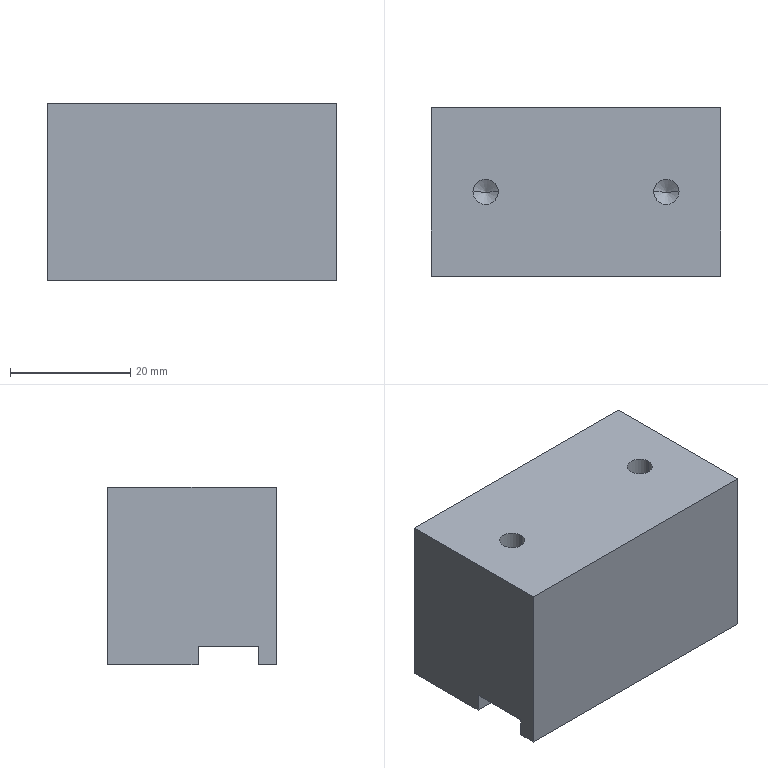Part | NX | features BREP 1 | 1 solid | 26 faces | box 48 x 28 x 29.5 mm | volume 37409 mm3 | plane 10 | cylinder 8 | cone 8 | commonest cylinder face diameters 4.2 x8
STEP:
#1=CARTESIAN_POINT('',(-17.1,0.,0.));
#2=VERTEX_POINT('',#1);
#3=CARTESIAN_POINT('',(-17.1,0.,-14.));
#4=VERTEX_POINT('',#3);
#5=CARTESIAN_POINT('',(-17.1,0.,0.));
#6=DIRECTION('',(0.,0.,1.));
#7=VECTOR('',#6,1000.);
#8=LINE('',#5,#7);
#9=EDGE_CURVE('',#2,#4,#8,.F.);
#10=ORIENTED_EDGE('',*,*,#9,.T.);
#11=CARTESIAN_POINT('',(-12.9,0.,-14.));
#12=VERTEX_POINT('',#11);
#13=CARTESIAN_POINT('',(-15.,0.,-14.));
#14=DIRECTION('',(0.,0.,1.));
#15=DIRECTION('',(1.,0.,0.));
#16=AXIS2_PLACEMENT_3D('',#13,#14,#15);
#17=CIRCLE('',#16,2.1);
#18=EDGE_CURVE('',#12,#4,#17,.T.);
#19=ORIENTED_EDGE('',*,*,#18,.F.);
#20=CARTESIAN_POINT('',(-12.9,0.,0.));
#21=VERTEX_POINT('',#20);
#22=CARTESIAN_POINT('',(-12.9,0.,0.));
#23=DIRECTION('',(0.,0.,1.));
#24=VECTOR('',#23,1000.);
#25=LINE('',#22,#24);
#26=EDGE_CURVE('',#21,#12,#25,.F.);
#27=ORIENTED_EDGE('',*,*,#26,.F.);
#28=CARTESIAN_POINT('',(-15.,0.,0.));
#29=DIRECTION('',(0.,0.,1.));
#30=DIRECTION('',(1.,0.,0.));
#31=AXIS2_PLACEMENT_3D('',#28,#29,#30);
#32=CIRCLE('',#31,2.1);
#33=EDGE_CURVE('',#21,#2,#32,.T.);
#34=ORIENTED_EDGE('',*,*,#33,.T.);
#35=EDGE_LOOP('',(#10,#19,#27,#34));
#36=FACE_BOUND('',#35,.T.);
#37=CARTESIAN_POINT('',(-15.,0.,0.));
#38=DIRECTION('',(0.,0.,1.));
#39=DIRECTION('',(1.,0.,0.));
#40=AXIS2_PLACEMENT_3D('',#37,#38,#39);
#41=CYLINDRICAL_SURFACE('',#40,2.1);
#42=ADVANCED_FACE('',(#36),#41,.F.);
#43=CARTESIAN_POINT('',(-15.,0.,-15.262));
#44=VERTEX_POINT('',#43);
#45=CARTESIAN_POINT('',(-17.1,0.,-14.));
#46=DIRECTION('',(-0.8572,0.,0.515));
#47=VECTOR('',#46,1000.);
#48=LINE('',#45,#47);
#49=EDGE_CURVE('',#44,#4,#48,.T.);
#50=ORIENTED_EDGE('',*,*,#49,.F.);
#51=CARTESIAN_POINT('',(-12.9,0.,-14.));
#52=DIRECTION('',(0.8572,0.,0.515));
#53=VECTOR('',#52,1000.);
#54=LINE('',#51,#53);
#55=EDGE_CURVE('',#44,#12,#54,.T.);
#56=ORIENTED_EDGE('',*,*,#55,.T.);
#57=ORIENTED_EDGE('',*,*,#18,.T.);
#58=EDGE_LOOP('',(#50,#56,#57));
#59=FACE_BOUND('',#58,.T.);
#60=CARTESIAN_POINT('',(-15.,0.,-14.));
#61=DIRECTION('',(0.,0.,1.));
#62=DIRECTION('',(1.,0.,0.));
#63=AXIS2_PLACEMENT_3D('',#60,#61,#62);
#64=CONICAL_SURFACE('',#63,2.1,1.03);
#65=ADVANCED_FACE('',(#59),#64,.F.);
#66=CARTESIAN_POINT('',(12.9,0.,0.));
#67=VERTEX_POINT('',#66);
#68=CARTESIAN_POINT('',(12.9,0.,-14.));
#69=VERTEX_POINT('',#68);
#70=CARTESIAN_POINT('',(12.9,0.,0.));
#71=DIRECTION('',(0.,0.,1.));
#72=VECTOR('',#71,1000.);
#73=LINE('',#70,#72);
#74=EDGE_CURVE('',#67,#69,#73,.F.);
#75=ORIENTED_EDGE('',*,*,#74,.T.);
#76=CARTESIAN_POINT('',(17.1,0.,-14.));
#77=VERTEX_POINT('',#76);
#78=CARTESIAN_POINT('',(15.,0.,-14.));
#79=DIRECTION('',(0.,0.,1.));
#80=DIRECTION('',(1.,0.,0.));
#81=AXIS2_PLACEMENT_3D('',#78,#79,#80);
#82=CIRCLE('',#81,2.1);
#83=EDGE_CURVE('',#77,#69,#82,.T.);
#84=ORIENTED_EDGE('',*,*,#83,.F.);
#85=CARTESIAN_POINT('',(17.1,0.,0.));
#86=VERTEX_POINT('',#85);
#87=CARTESIAN_POINT('',(17.1,0.,0.));
#88=DIRECTION('',(0.,0.,1.));
#89=VECTOR('',#88,1000.);
#90=LINE('',#87,#89);
#91=EDGE_CURVE('',#86,#77,#90,.F.);
#92=ORIENTED_EDGE('',*,*,#91,.F.);
#93=CARTESIAN_POINT('',(15.,0.,0.));
#94=DIRECTION('',(0.,0.,1.));
#95=DIRECTION('',(1.,0.,0.));
#96=AXIS2_PLACEMENT_3D('',#93,#94,#95);
#97=CIRCLE('',#96,2.1);
#98=EDGE_CURVE('',#86,#67,#97,.T.);
#99=ORIENTED_EDGE('',*,*,#98,.T.);
#100=EDGE_LOOP('',(#75,#84,#92,#99));
#101=FACE_BOUND('',#100,.T.);
#102=CARTESIAN_POINT('',(15.,0.,0.));
#103=DIRECTION('',(0.,0.,1.));
#104=DIRECTION('',(1.,0.,0.));
#105=AXIS2_PLACEMENT_3D('',#102,#103,#104);
#106=CYLINDRICAL_SURFACE('',#105,2.1);
#107=ADVANCED_FACE('',(#101),#106,.F.);
#108=CARTESIAN_POINT('',(15.,0.,-15.262));
#109=VERTEX_POINT('',#108);
#110=CARTESIAN_POINT('',(12.9,0.,-14.));
#111=DIRECTION('',(-0.8572,0.,0.515));
#112=VECTOR('',#111,1000.);
#113=LINE('',#110,#112);
#114=EDGE_CURVE('',#109,#69,#113,.T.);
#115=ORIENTED_EDGE('',*,*,#114,.F.);
#116=CARTESIAN_POINT('',(17.1,0.,-14.));
#117=DIRECTION('',(0.8572,0.,0.515));
#118=VECTOR('',#117,1000.);
#119=LINE('',#116,#118);
#120=EDGE_CURVE('',#109,#77,#119,.T.);
#121=ORIENTED_EDGE('',*,*,#120,.T.);
#122=ORIENTED_EDGE('',*,*,#83,.T.);
#123=EDGE_LOOP('',(#115,#121,#122));
#124=FACE_BOUND('',#123,.T.);
#125=CARTESIAN_POINT('',(15.,0.,-14.));
#126=DIRECTION('',(0.,0.,1.));
#127=DIRECTION('',(1.,0.,0.));
#128=AXIS2_PLACEMENT_3D('',#125,#126,#127);
#129=CONICAL_SURFACE('',#128,2.1,1.03);
#130=ADVANCED_FACE('',(#124),#129,.F.);
#131=CARTESIAN_POINT('',(17.1,7.35,-15.5));
#132=VERTEX_POINT('',#131);
#133=CARTESIAN_POINT('',(17.1,7.35,-29.5));
#134=VERTEX_POINT('',#133);
#135=CARTESIAN_POINT('',(17.1,7.35,-29.5));
#136=DIRECTION('',(0.,0.,-1.));
#137=VECTOR('',#136,1000.);
#138=LINE('',#135,#137);
#139=EDGE_CURVE('',#132,#134,#138,.T.);
#140=ORIENTED_EDGE('',*,*,#139,.F.);
#141=CARTESIAN_POINT('',(12.9,7.35,-15.5));
#142=VERTEX_POINT('',#141);
#143=CARTESIAN_POINT('',(15.,7.35,-15.5));
#144=DIRECTION('',(0.,0.,-1.));
#145=DIRECTION('',(-1.,0.,0.));
#146=AXIS2_PLACEMENT_3D('',#143,#144,#145);
#147=CIRCLE('',#146,2.1);
#148=EDGE_CURVE('',#142,#132,#147,.T.);
#149=ORIENTED_EDGE('',*,*,#148,.F.);
#150=CARTESIAN_POINT('',(12.9,7.35,-29.5));
#151=VERTEX_POINT('',#150);
#152=CARTESIAN_POINT('',(12.9,7.35,-29.5));
#153=DIRECTION('',(0.,0.,-1.));
#154=VECTOR('',#153,1000.);
#155=LINE('',#152,#154);
#156=EDGE_CURVE('',#142,#151,#155,.T.);
#157=ORIENTED_EDGE('',*,*,#156,.T.);
#158=CARTESIAN_POINT('',(15.,7.35,-29.5));
#159=DIRECTION('',(0.,0.,-1.));
#160=DIRECTION('',(-1.,0.,0.));
#161=AXIS2_PLACEMENT_3D('',#158,#159,#160);
#162=CIRCLE('',#161,2.1);
#163=EDGE_CURVE('',#151,#134,#162,.T.);
#164=ORIENTED_EDGE('',*,*,#163,.T.);
#165=EDGE_LOOP('',(#140,#149,#157,#164));
#166=FACE_BOUND('',#165,.T.);
#167=CARTESIAN_POINT('',(15.,7.35,-29.5));
#168=DIRECTION('',(0.,0.,-1.));
#169=DIRECTION('',(-1.,0.,0.));
#170=AXIS2_PLACEMENT_3D('',#167,#168,#169);
#171=CYLINDRICAL_SURFACE('',#170,2.1);
#172=ADVANCED_FACE('',(#166),#171,.F.);
#173=CARTESIAN_POINT('',(15.,7.35,-14.238));
#174=VERTEX_POINT('',#173);
#175=CARTESIAN_POINT('',(17.1,7.35,-15.5));
#176=DIRECTION('',(0.8572,0.,-0.515));
#177=VECTOR('',#176,1000.);
#178=LINE('',#175,#177);
#179=EDGE_CURVE('',#132,#174,#178,.F.);
#180=ORIENTED_EDGE('',*,*,#179,.T.);
#181=CARTESIAN_POINT('',(12.9,7.35,-15.5));
#182=DIRECTION('',(-0.8572,0.,-0.515));
#183=VECTOR('',#182,1000.);
#184=LINE('',#181,#183);
#185=EDGE_CURVE('',#142,#174,#184,.F.);
#186=ORIENTED_EDGE('',*,*,#185,.F.);
#187=ORIENTED_EDGE('',*,*,#148,.T.);
#188=EDGE_LOOP('',(#180,#186,#187));
#189=FACE_BOUND('',#188,.T.);
#190=CARTESIAN_POINT('',(15.,7.35,-15.5));
#191=DIRECTION('',(0.,0.,-1.));
#192=DIRECTION('',(-1.,0.,0.));
#193=AXIS2_PLACEMENT_3D('',#190,#191,#192);
#194=CONICAL_SURFACE('',#193,2.1,1.03);
#195=ADVANCED_FACE('',(#189),#194,.F.);
#196=CARTESIAN_POINT('',(-12.9,7.35,-15.5));
#197=VERTEX_POINT('',#196);
#198=CARTESIAN_POINT('',(-12.9,7.35,-29.5));
#199=VERTEX_POINT('',#198);
#200=CARTESIAN_POINT('',(-12.9,7.35,-29.5));
#201=DIRECTION('',(0.,0.,-1.));
#202=VECTOR('',#201,1000.);
#203=LINE('',#200,#202);
#204=EDGE_CURVE('',#197,#199,#203,.T.);
#205=ORIENTED_EDGE('',*,*,#204,.F.);
#206=CARTESIAN_POINT('',(-17.1,7.35,-15.5));
#207=VERTEX_POINT('',#206);
#208=CARTESIAN_POINT('',(-15.,7.35,-15.5));
#209=DIRECTION('',(0.,0.,-1.));
#210=DIRECTION('',(-1.,0.,0.));
#211=AXIS2_PLACEMENT_3D('',#208,#209,#210);
#212=CIRCLE('',#211,2.1);
#213=EDGE_CURVE('',#207,#197,#212,.T.);
#214=ORIENTED_EDGE('',*,*,#213,.F.);
#215=CARTESIAN_POINT('',(-17.1,7.35,-29.5));
#216=VERTEX_POINT('',#215);
#217=CARTESIAN_POINT('',(-17.1,7.35,-29.5));
#218=DIRECTION('',(0.,0.,-1.));
#219=VECTOR('',#218,1000.);
#220=LINE('',#217,#219);
#221=EDGE_CURVE('',#207,#216,#220,.T.);
#222=ORIENTED_EDGE('',*,*,#221,.T.);
#223=CARTESIAN_POINT('',(-15.,7.35,-29.5));
#224=DIRECTION('',(0.,0.,-1.));
#225=DIRECTION('',(-1.,0.,0.));
#226=AXIS2_PLACEMENT_3D('',#223,#224,#225);
#227=CIRCLE('',#226,2.1);
#228=EDGE_CURVE('',#216,#199,#227,.T.);
#229=ORIENTED_EDGE('',*,*,#228,.T.);
#230=EDGE_LOOP('',(#205,#214,#222,#229));
#231=FACE_BOUND('',#230,.T.);
#232=CARTESIAN_POINT('',(-15.,7.35,-29.5));
#233=DIRECTION('',(0.,0.,-1.));
#234=DIRECTION('',(-1.,0.,0.));
#235=AXIS2_PLACEMENT_3D('',#232,#233,#234);
#236=CYLINDRICAL_SURFACE('',#235,2.1);
#237=ADVANCED_FACE('',(#231),#236,.F.);
#238=CARTESIAN_POINT('',(-15.,7.35,-14.238));
#239=VERTEX_POINT('',#238);
#240=CARTESIAN_POINT('',(-12.9,7.35,-15.5));
#241=DIRECTION('',(0.8572,0.,-0.515));
#242=VECTOR('',#241,1000.);
#243=LINE('',#240,#242);
#244=EDGE_CURVE('',#197,#239,#243,.F.);
#245=ORIENTED_EDGE('',*,*,#244,.T.);
#246=CARTESIAN_POINT('',(-17.1,7.35,-15.5));
#247=DIRECTION('',(-0.8572,0.,-0.515));
#248=VECTOR('',#247,1000.);
#249=LINE('',#246,#248);
#250=EDGE_CURVE('',#207,#239,#249,.F.);
#251=ORIENTED_EDGE('',*,*,#250,.F.);
#252=ORIENTED_EDGE('',*,*,#213,.T.);
#253=EDGE_LOOP('',(#245,#251,#252));
#254=FACE_BOUND('',#253,.T.);
#255=CARTESIAN_POINT('',(-15.,7.35,-15.5));
#256=DIRECTION('',(0.,0.,-1.));
#257=DIRECTION('',(-1.,0.,0.));
#258=AXIS2_PLACEMENT_3D('',#255,#256,#257);
#259=CONICAL_SURFACE('',#258,2.1,1.03);
#260=ADVANCED_FACE('',(#254),#259,.F.);
#261=CARTESIAN_POINT('',(24.,-11.,-26.5));
#262=VERTEX_POINT('',#261);
#263=CARTESIAN_POINT('',(24.,-11.,-29.5));
#264=VERTEX_POINT('',#263);
#265=CARTESIAN_POINT('',(24.,-11.,-26.5));
#266=DIRECTION('',(0.,0.,-1.));
#267=VECTOR('',#266,1000.);
#268=LINE('',#265,#267);
#269=EDGE_CURVE('',#262,#264,#268,.T.);
#270=ORIENTED_EDGE('',*,*,#269,.T.);
#271=CARTESIAN_POINT('',(-24.,-11.,-29.5));
#272=VERTEX_POINT('',#271);
#273=CARTESIAN_POINT('',(-24.,-11.,-29.5));
#274=DIRECTION('',(1.,0.,0.));
#275=VECTOR('',#274,1000.);
#276=LINE('',#273,#275);
#277=EDGE_CURVE('',#272,#264,#276,.T.);
#278=ORIENTED_EDGE('',*,*,#277,.F.);
#279=CARTESIAN_POINT('',(-24.,-11.,-26.5));
#280=VERTEX_POINT('',#279);
#281=CARTESIAN_POINT('',(-24.,-11.,-26.5));
#282=DIRECTION('',(0.,0.,-1.));
#283=VECTOR('',#282,1000.);
#284=LINE('',#281,#283);
#285=EDGE_CURVE('',#280,#272,#284,.T.);
#286=ORIENTED_EDGE('',*,*,#285,.F.);
#287=CARTESIAN_POINT('',(-24.,-11.,-26.5));
#288=DIRECTION('',(1.,0.,0.));
#289=VECTOR('',#288,1000.);
#290=LINE('',#287,#289);
#291=EDGE_CURVE('',#280,#262,#290,.T.);
#292=ORIENTED_EDGE('',*,*,#291,.T.);
#293=EDGE_LOOP('',(#270,#278,#286,#292));
#294=FACE_BOUND('',#293,.T.);
#295=CARTESIAN_POINT('',(-24.,-11.,-26.5));
#296=DIRECTION('',(0.,-1.,0.));
#297=DIRECTION('',(0.,0.,-1.));
#298=AXIS2_PLACEMENT_3D('',#295,#296,#297);
#299=PLANE('',#298);
#300=ADVANCED_FACE('',(#294),#299,.F.);
#301=CARTESIAN_POINT('',(24.,-1.,-29.5));
#302=VERTEX_POINT('',#301);
#303=CARTESIAN_POINT('',(24.,-1.,-26.5));
#304=VERTEX_POINT('',#303);
#305=CARTESIAN_POINT('',(24.,-1.,-26.5));
#306=DIRECTION('',(0.,0.,1.));
#307=VECTOR('',#306,1000.);
#308=LINE('',#305,#307);
#309=EDGE_CURVE('',#302,#304,#308,.T.);
#310=ORIENTED_EDGE('',*,*,#309,.T.);
#311=CARTESIAN_POINT('',(-24.,-1.,-26.5));
#312=VERTEX_POINT('',#311);
#313=CARTESIAN_POINT('',(-24.,-1.,-26.5));
#314=DIRECTION('',(1.,0.,0.));
#315=VECTOR('',#314,1000.);
#316=LINE('',#313,#315);
#317=EDGE_CURVE('',#312,#304,#316,.T.);
#318=ORIENTED_EDGE('',*,*,#317,.F.);
#319=CARTESIAN_POINT('',(-24.,-1.,-29.5));
#320=VERTEX_POINT('',#319);
#321=CARTESIAN_POINT('',(-24.,-1.,-26.5));
#322=DIRECTION('',(0.,0.,1.));
#323=VECTOR('',#322,1000.);
#324=LINE('',#321,#323);
#325=EDGE_CURVE('',#320,#312,#324,.T.);
#326=ORIENTED_EDGE('',*,*,#325,.F.);
#327=CARTESIAN_POINT('',(-24.,-1.,-29.5));
#328=DIRECTION('',(1.,0.,0.));
#329=VECTOR('',#328,1000.);
#330=LINE('',#327,#329);
#331=EDGE_CURVE('',#320,#302,#330,.T.);
#332=ORIENTED_EDGE('',*,*,#331,.T.);
#333=EDGE_LOOP('',(#310,#318,#326,#332));
#334=FACE_BOUND('',#333,.T.);
#335=CARTESIAN_POINT('',(-24.,-1.,-26.5));
#336=DIRECTION('',(0.,1.,0.));
#337=DIRECTION('',(0.,0.,1.));
#338=AXIS2_PLACEMENT_3D('',#335,#336,#337);
#339=PLANE('',#338);
#340=ADVANCED_FACE('',(#334),#339,.F.);
#341=CARTESIAN_POINT('',(24.,-1.,-26.5));
#342=DIRECTION('',(0.,-1.,0.));
#343=VECTOR('',#342,1000.);
#344=LINE('',#341,#343);
#345=EDGE_CURVE('',#304,#262,#344,.T.);
#346=ORIENTED_EDGE('',*,*,#345,.T.);
#347=ORIENTED_EDGE('',*,*,#291,.F.);
#348=CARTESIAN_POINT('',(-24.,-1.,-26.5));
#349=DIRECTION('',(0.,-1.,0.));
#350=VECTOR('',#349,1000.);
#351=LINE('',#348,#350);
#352=EDGE_CURVE('',#312,#280,#351,.T.);
#353=ORIENTED_EDGE('',*,*,#352,.F.);
#354=ORIENTED_EDGE('',*,*,#317,.T.);
#355=EDGE_LOOP('',(#346,#347,#353,#354));
#356=FACE_BOUND('',#355,.T.);
#357=CARTESIAN_POINT('',(-24.,-1.,-26.5));
#358=DIRECTION('',(0.,0.,1.));
#359=DIRECTION('',(1.,0.,0.));
#360=AXIS2_PLACEMENT_3D('',#357,#358,#359);
#361=PLANE('',#360);
#362=ADVANCED_FACE('',(#356),#361,.F.);
#363=CARTESIAN_POINT('',(-24.,14.,-29.5));
#364=VERTEX_POINT('',#363);
#365=CARTESIAN_POINT('',(-24.,14.,-29.5));
#366=DIRECTION('',(0.,1.,0.));
#367=VECTOR('',#366,1000.);
#368=LINE('',#365,#367);
#369=EDGE_CURVE('',#320,#364,#368,.T.);
#370=ORIENTED_EDGE('',*,*,#369,.F.);
#371=ORIENTED_EDGE('',*,*,#325,.T.);
#372=ORIENTED_EDGE('',*,*,#352,.T.);
#373=ORIENTED_EDGE('',*,*,#285,.T.);
#374=CARTESIAN_POINT('',(-24.,-14.,-29.5));
#375=VERTEX_POINT('',#374);
#376=CARTESIAN_POINT('',(-24.,14.,-29.5));
#377=DIRECTION('',(0.,1.,0.));
#378=VECTOR('',#377,1000.);
#379=LINE('',#376,#378);
#380=EDGE_CURVE('',#375,#272,#379,.T.);
#381=ORIENTED_EDGE('',*,*,#380,.F.);
#382=CARTESIAN_POINT('',(-24.,-14.,0.));
#383=VERTEX_POINT('',#382);
#384=CARTESIAN_POINT('',(-24.,-14.,0.));
#385=DIRECTION('',(0.,0.,-1.));
#386=VECTOR('',#385,1000.);
#387=LINE('',#384,#386);
#388=EDGE_CURVE('',#383,#375,#387,.T.);
#389=ORIENTED_EDGE('',*,*,#388,.F.);
#390=CARTESIAN_POINT('',(-24.,14.,0.));
#391=VERTEX_POINT('',#390);
#392=CARTESIAN_POINT('',(-24.,14.,0.));
#393=DIRECTION('',(0.,-1.,0.));
#394=VECTOR('',#393,1000.);
#395=LINE('',#392,#394);
#396=EDGE_CURVE('',#391,#383,#395,.T.);
#397=ORIENTED_EDGE('',*,*,#396,.F.);
#398=CARTESIAN_POINT('',(-24.,14.,0.));
#399=DIRECTION('',(0.,0.,1.));
#400=VECTOR('',#399,1000.);
#401=LINE('',#398,#400);
#402=EDGE_CURVE('',#364,#391,#401,.T.);
#403=ORIENTED_EDGE('',*,*,#402,.F.);
#404=EDGE_LOOP('',(#370,#371,#372,#373,#381,#389,#397,#403));
#405=FACE_BOUND('',#404,.T.);
#406=CARTESIAN_POINT('',(-24.,0.,0.));
#407=DIRECTION('',(1.,0.,0.));
#408=DIRECTION('',(0.,0.,-1.));
#409=AXIS2_PLACEMENT_3D('',#406,#407,#408);
#410=PLANE('',#409);
#411=ADVANCED_FACE('',(#405),#410,.F.);
#412=ORIENTED_EDGE('',*,*,#309,.F.);
#413=CARTESIAN_POINT('',(24.,14.,-29.5));
#414=VERTEX_POINT('',#413);
#415=CARTESIAN_POINT('',(24.,14.,-29.5));
#416=DIRECTION('',(0.,1.,0.));
#417=VECTOR('',#416,1000.);
#418=LINE('',#415,#417);
#419=EDGE_CURVE('',#302,#414,#418,.T.);
#420=ORIENTED_EDGE('',*,*,#419,.T.);
#421=CARTESIAN_POINT('',(24.,14.,0.));
#422=VERTEX_POINT('',#421);
#423=CARTESIAN_POINT('',(24.,14.,0.));
#424=DIRECTION('',(0.,0.,1.));
#425=VECTOR('',#424,1000.);
#426=LINE('',#423,#425);
#427=EDGE_CURVE('',#414,#422,#426,.T.);
#428=ORIENTED_EDGE('',*,*,#427,.T.);
#429=CARTESIAN_POINT('',(24.,-14.,0.));
#430=VERTEX_POINT('',#429);
#431=CARTESIAN_POINT('',(24.,14.,0.));
#432=DIRECTION('',(0.,-1.,0.));
#433=VECTOR('',#432,1000.);
#434=LINE('',#431,#433);
#435=EDGE_CURVE('',#422,#430,#434,.T.);
#436=ORIENTED_EDGE('',*,*,#435,.T.);
#437=CARTESIAN_POINT('',(24.,-14.,-29.5));
#438=VERTEX_POINT('',#437);
#439=CARTESIAN_POINT('',(24.,-14.,0.));
#440=DIRECTION('',(0.,0.,-1.));
#441=VECTOR('',#440,1000.);
#442=LINE('',#439,#441);
#443=EDGE_CURVE('',#430,#438,#442,.T.);
#444=ORIENTED_EDGE('',*,*,#443,.T.);
#445=CARTESIAN_POINT('',(24.,14.,-29.5));
#446=DIRECTION('',(0.,1.,0.));
#447=VECTOR('',#446,1000.);
#448=LINE('',#445,#447);
#449=EDGE_CURVE('',#438,#264,#448,.T.);
#450=ORIENTED_EDGE('',*,*,#449,.T.);
#451=ORIENTED_EDGE('',*,*,#269,.F.);
#452=ORIENTED_EDGE('',*,*,#345,.F.);
#453=EDGE_LOOP('',(#412,#420,#428,#436,#444,#450,#451,#452));
#454=FACE_BOUND('',#453,.T.);
#455=CARTESIAN_POINT('',(24.,0.,0.));
#456=DIRECTION('',(1.,0.,0.));
#457=DIRECTION('',(0.,0.,-1.));
#458=AXIS2_PLACEMENT_3D('',#455,#456,#457);
#459=PLANE('',#458);
#460=ADVANCED_FACE('',(#454),#459,.T.);
#461=ORIENTED_EDGE('',*,*,#402,.T.);
#462=CARTESIAN_POINT('',(24.,14.,0.));
#463=DIRECTION('',(-1.,0.,0.));
#464=VECTOR('',#463,1000.);
#465=LINE('',#462,#464);
#466=EDGE_CURVE('',#422,#391,#465,.T.);
#467=ORIENTED_EDGE('',*,*,#466,.F.);
#468=ORIENTED_EDGE('',*,*,#427,.F.);
#469=CARTESIAN_POINT('',(24.,14.,-29.5));
#470=DIRECTION('',(-1.,0.,0.));
#471=VECTOR('',#470,1000.);
#472=LINE('',#469,#471);
#473=EDGE_CURVE('',#414,#364,#472,.T.);
#474=ORIENTED_EDGE('',*,*,#473,.T.);
#475=EDGE_LOOP('',(#461,#467,#468,#474));
#476=FACE_BOUND('',#475,.T.);
#477=CARTESIAN_POINT('',(24.,14.,0.));
#478=DIRECTION('',(0.,-1.,0.));
#479=DIRECTION('',(0.,0.,-1.));
#480=AXIS2_PLACEMENT_3D('',#477,#478,#479);
#481=PLANE('',#480);
#482=ADVANCED_FACE('',(#476),#481,.F.);
#483=ORIENTED_EDGE('',*,*,#380,.T.);
#484=ORIENTED_EDGE('',*,*,#277,.T.);
#485=ORIENTED_EDGE('',*,*,#449,.F.);
#486=CARTESIAN_POINT('',(24.,-14.,-29.5));
#487=DIRECTION('',(-1.,0.,0.));
#488=VECTOR('',#487,1000.);
#489=LINE('',#486,#488);
#490=EDGE_CURVE('',#438,#375,#489,.T.);
#491=ORIENTED_EDGE('',*,*,#490,.T.);
#492=EDGE_LOOP('',(#483,#484,#485,#491));
#493=FACE_BOUND('',#492,.T.);
#494=CARTESIAN_POINT('',(24.,14.,-29.5));
#495=DIRECTION('',(0.,0.,1.));
#496=DIRECTION('',(1.,0.,0.));
#497=AXIS2_PLACEMENT_3D('',#494,#495,#496);
#498=PLANE('',#497);
#499=ADVANCED_FACE('',(#493),#498,.F.);
#500=ORIENTED_EDGE('',*,*,#388,.T.);
#501=ORIENTED_EDGE('',*,*,#490,.F.);
#502=ORIENTED_EDGE('',*,*,#443,.F.);
#503=CARTESIAN_POINT('',(24.,-14.,0.));
#504=DIRECTION('',(-1.,0.,0.));
#505=VECTOR('',#504,1000.);
#506=LINE('',#503,#505);
#507=EDGE_CURVE('',#430,#383,#506,.T.);
#508=ORIENTED_EDGE('',*,*,#507,.T.);
#509=EDGE_LOOP('',(#500,#501,#502,#508));
#510=FACE_BOUND('',#509,.T.);
#511=CARTESIAN_POINT('',(24.,-14.,0.));
#512=DIRECTION('',(0.,1.,0.));
#513=DIRECTION('',(0.,0.,1.));
#514=AXIS2_PLACEMENT_3D('',#511,#512,#513);
#515=PLANE('',#514);
#516=ADVANCED_FACE('',(#510),#515,.F.);
#517=ORIENTED_EDGE('',*,*,#396,.T.);
#518=ORIENTED_EDGE('',*,*,#507,.F.);
#519=ORIENTED_EDGE('',*,*,#435,.F.);
#520=ORIENTED_EDGE('',*,*,#466,.T.);
#521=EDGE_LOOP('',(#517,#518,#519,#520));
#522=FACE_BOUND('',#521,.T.);
#523=ORIENTED_EDGE('',*,*,#98,.F.);
#524=CARTESIAN_POINT('',(15.,0.,0.));
#525=DIRECTION('',(0.,0.,1.));
#526=DIRECTION('',(1.,0.,0.));
#527=AXIS2_PLACEMENT_3D('',#524,#525,#526);
#528=CIRCLE('',#527,2.1);
#529=EDGE_CURVE('',#67,#86,#528,.T.);
#530=ORIENTED_EDGE('',*,*,#529,.F.);
#531=EDGE_LOOP('',(#523,#530));
#532=FACE_BOUND('',#531,.T.);
#533=ORIENTED_EDGE('',*,*,#33,.F.);
#534=CARTESIAN_POINT('',(-15.,0.,0.));
#535=DIRECTION('',(0.,0.,1.));
#536=DIRECTION('',(1.,0.,0.));
#537=AXIS2_PLACEMENT_3D('',#534,#535,#536);
#538=CIRCLE('',#537,2.1);
#539=EDGE_CURVE('',#2,#21,#538,.T.);
#540=ORIENTED_EDGE('',*,*,#539,.F.);
#541=EDGE_LOOP('',(#533,#540));
#542=FACE_BOUND('',#541,.T.);
#543=CARTESIAN_POINT('',(24.,14.,0.));
#544=DIRECTION('',(0.,0.,-1.));
#545=DIRECTION('',(-1.,0.,0.));
#546=AXIS2_PLACEMENT_3D('',#543,#544,#545);
#547=PLANE('',#546);
#548=ADVANCED_FACE('',(#522,#532,#542),#547,.F.);
#549=ORIENTED_EDGE('',*,*,#419,.F.);
#550=ORIENTED_EDGE('',*,*,#331,.F.);
#551=ORIENTED_EDGE('',*,*,#369,.T.);
#552=ORIENTED_EDGE('',*,*,#473,.F.);
#553=EDGE_LOOP('',(#549,#550,#551,#552));
#554=FACE_BOUND('',#553,.T.);
#555=ORIENTED_EDGE('',*,*,#228,.F.);
#556=CARTESIAN_POINT('',(-15.,7.35,-29.5));
#557=DIRECTION('',(0.,0.,-1.));
#558=DIRECTION('',(-1.,0.,0.));
#559=AXIS2_PLACEMENT_3D('',#556,#557,#558);
#560=CIRCLE('',#559,2.1);
#561=EDGE_CURVE('',#199,#216,#560,.T.);
#562=ORIENTED_EDGE('',*,*,#561,.F.);
#563=EDGE_LOOP('',(#555,#562));
#564=FACE_BOUND('',#563,.T.);
#565=ORIENTED_EDGE('',*,*,#163,.F.);
#566=CARTESIAN_POINT('',(15.,7.35,-29.5));
#567=DIRECTION('',(0.,0.,-1.));
#568=DIRECTION('',(-1.,0.,0.));
#569=AXIS2_PLACEMENT_3D('',#566,#567,#568);
#570=CIRCLE('',#569,2.1);
#571=EDGE_CURVE('',#134,#151,#570,.T.);
#572=ORIENTED_EDGE('',*,*,#571,.F.);
#573=EDGE_LOOP('',(#565,#572));
#574=FACE_BOUND('',#573,.T.);
#575=CARTESIAN_POINT('',(24.,14.,-29.5));
#576=DIRECTION('',(0.,0.,1.));
#577=DIRECTION('',(1.,0.,0.));
#578=AXIS2_PLACEMENT_3D('',#575,#576,#577);
#579=PLANE('',#578);
#580=ADVANCED_FACE('',(#554,#564,#574),#579,.F.);
#581=ORIENTED_EDGE('',*,*,#250,.T.);
#582=ORIENTED_EDGE('',*,*,#244,.F.);
#583=CARTESIAN_POINT('',(-15.,7.35,-15.5));
#584=DIRECTION('',(0.,0.,-1.));
#585=DIRECTION('',(-1.,0.,0.));
#586=AXIS2_PLACEMENT_3D('',#583,#584,#585);
#587=CIRCLE('',#586,2.1);
#588=EDGE_CURVE('',#197,#207,#587,.T.);
#589=ORIENTED_EDGE('',*,*,#588,.T.);
#590=EDGE_LOOP('',(#581,#582,#589));
#591=FACE_BOUND('',#590,.T.);
#592=CARTESIAN_POINT('',(-15.,7.35,-15.5));
#593=DIRECTION('',(0.,0.,-1.));
#594=DIRECTION('',(-1.,0.,0.));
#595=AXIS2_PLACEMENT_3D('',#592,#593,#594);
#596=CONICAL_SURFACE('',#595,2.1,1.03);
#597=ADVANCED_FACE('',(#591),#596,.F.);
#598=ORIENTED_EDGE('',*,*,#588,.F.);
#599=ORIENTED_EDGE('',*,*,#204,.T.);
#600=ORIENTED_EDGE('',*,*,#561,.T.);
#601=ORIENTED_EDGE('',*,*,#221,.F.);
#602=EDGE_LOOP('',(#598,#599,#600,#601));
#603=FACE_BOUND('',#602,.T.);
#604=CARTESIAN_POINT('',(-15.,7.35,-29.5));
#605=DIRECTION('',(0.,0.,-1.));
#606=DIRECTION('',(-1.,0.,0.));
#607=AXIS2_PLACEMENT_3D('',#604,#605,#606);
#608=CYLINDRICAL_SURFACE('',#607,2.1);
#609=ADVANCED_FACE('',(#603),#608,.F.);
#610=ORIENTED_EDGE('',*,*,#185,.T.);
#611=ORIENTED_EDGE('',*,*,#179,.F.);
#612=CARTESIAN_POINT('',(15.,7.35,-15.5));
#613=DIRECTION('',(0.,0.,-1.));
#614=DIRECTION('',(-1.,0.,0.));
#615=AXIS2_PLACEMENT_3D('',#612,#613,#614);
#616=CIRCLE('',#615,2.1);
#617=EDGE_CURVE('',#132,#142,#616,.T.);
#618=ORIENTED_EDGE('',*,*,#617,.T.);
#619=EDGE_LOOP('',(#610,#611,#618));
#620=FACE_BOUND('',#619,.T.);
#621=CARTESIAN_POINT('',(15.,7.35,-15.5));
#622=DIRECTION('',(0.,0.,-1.));
#623=DIRECTION('',(-1.,0.,0.));
#624=AXIS2_PLACEMENT_3D('',#621,#622,#623);
#625=CONICAL_SURFACE('',#624,2.1,1.03);
#626=ADVANCED_FACE('',(#620),#625,.F.);
#627=ORIENTED_EDGE('',*,*,#617,.F.);
#628=ORIENTED_EDGE('',*,*,#139,.T.);
#629=ORIENTED_EDGE('',*,*,#571,.T.);
#630=ORIENTED_EDGE('',*,*,#156,.F.);
#631=EDGE_LOOP('',(#627,#628,#629,#630));
#632=FACE_BOUND('',#631,.T.);
#633=CARTESIAN_POINT('',(15.,7.35,-29.5));
#634=DIRECTION('',(0.,0.,-1.));
#635=DIRECTION('',(-1.,0.,0.));
#636=AXIS2_PLACEMENT_3D('',#633,#634,#635);
#637=CYLINDRICAL_SURFACE('',#636,2.1);
#638=ADVANCED_FACE('',(#632),#637,.F.);
#639=ORIENTED_EDGE('',*,*,#120,.F.);
#640=ORIENTED_EDGE('',*,*,#114,.T.);
#641=CARTESIAN_POINT('',(15.,0.,-14.));
#642=DIRECTION('',(0.,0.,1.));
#643=DIRECTION('',(1.,0.,0.));
#644=AXIS2_PLACEMENT_3D('',#641,#642,#643);
#645=CIRCLE('',#644,2.1);
#646=EDGE_CURVE('',#69,#77,#645,.T.);
#647=ORIENTED_EDGE('',*,*,#646,.T.);
#648=EDGE_LOOP('',(#639,#640,#647));
#649=FACE_BOUND('',#648,.T.);
#650=CARTESIAN_POINT('',(15.,0.,-14.));
#651=DIRECTION('',(0.,0.,1.));
#652=DIRECTION('',(1.,0.,0.));
#653=AXIS2_PLACEMENT_3D('',#650,#651,#652);
#654=CONICAL_SURFACE('',#653,2.1,1.03);
#655=ADVANCED_FACE('',(#649),#654,.F.);
#656=ORIENTED_EDGE('',*,*,#646,.F.);
#657=ORIENTED_EDGE('',*,*,#74,.F.);
#658=ORIENTED_EDGE('',*,*,#529,.T.);
#659=ORIENTED_EDGE('',*,*,#91,.T.);
#660=EDGE_LOOP('',(#656,#657,#658,#659));
#661=FACE_BOUND('',#660,.T.);
#662=CARTESIAN_POINT('',(15.,0.,0.));
#663=DIRECTION('',(0.,0.,1.));
#664=DIRECTION('',(1.,0.,0.));
#665=AXIS2_PLACEMENT_3D('',#662,#663,#664);
#666=CYLINDRICAL_SURFACE('',#665,2.1);
#667=ADVANCED_FACE('',(#661),#666,.F.);
#668=ORIENTED_EDGE('',*,*,#55,.F.);
#669=ORIENTED_EDGE('',*,*,#49,.T.);
#670=CARTESIAN_POINT('',(-15.,0.,-14.));
#671=DIRECTION('',(0.,0.,1.));
#672=DIRECTION('',(1.,0.,0.));
#673=AXIS2_PLACEMENT_3D('',#670,#671,#672);
#674=CIRCLE('',#673,2.1);
#675=EDGE_CURVE('',#4,#12,#674,.T.);
#676=ORIENTED_EDGE('',*,*,#675,.T.);
#677=EDGE_LOOP('',(#668,#669,#676));
#678=FACE_BOUND('',#677,.T.);
#679=CARTESIAN_POINT('',(-15.,0.,-14.));
#680=DIRECTION('',(0.,0.,1.));
#681=DIRECTION('',(1.,0.,0.));
#682=AXIS2_PLACEMENT_3D('',#679,#680,#681);
#683=CONICAL_SURFACE('',#682,2.1,1.03);
#684=ADVANCED_FACE('',(#678),#683,.F.);
#685=ORIENTED_EDGE('',*,*,#675,.F.);
#686=ORIENTED_EDGE('',*,*,#9,.F.);
#687=ORIENTED_EDGE('',*,*,#539,.T.);
#688=ORIENTED_EDGE('',*,*,#26,.T.);
#689=EDGE_LOOP('',(#685,#686,#687,#688));
#690=FACE_BOUND('',#689,.T.);
#691=CARTESIAN_POINT('',(-15.,0.,0.));
#692=DIRECTION('',(0.,0.,1.));
#693=DIRECTION('',(1.,0.,0.));
#694=AXIS2_PLACEMENT_3D('',#691,#692,#693);
#695=CYLINDRICAL_SURFACE('',#694,2.1);
#696=ADVANCED_FACE('',(#690),#695,.F.);
#697=CLOSED_SHELL('',(#42,#65,#107,#130,#172,#195,#237,#260,#300,#340,#362,#411,#460,#482,#499,#516,#548,#580,#597,#609,#626,#638,#655,#667,#684,#696));
#698=MANIFOLD_SOLID_BREP('',#697);
#699=(LENGTH_UNIT()NAMED_UNIT(*)SI_UNIT(.MILLI.,.METRE.));
#700=UNCERTAINTY_MEASURE_WITH_UNIT(LENGTH_MEASURE(0.00001),#699,'','');
#701=(NAMED_UNIT(*)PLANE_ANGLE_UNIT()SI_UNIT($,.RADIAN.));
#702=(NAMED_UNIT(*)SI_UNIT($,.STERADIAN.)SOLID_ANGLE_UNIT());
#703=(GEOMETRIC_REPRESENTATION_CONTEXT(3)GLOBAL_UNCERTAINTY_ASSIGNED_CONTEXT((#700))GLOBAL_UNIT_ASSIGNED_CONTEXT((#699,#701,#702))REPRESENTATION_CONTEXT('',''));
#704=ADVANCED_BREP_SHAPE_REPRESENTATION('',(#698),#703);